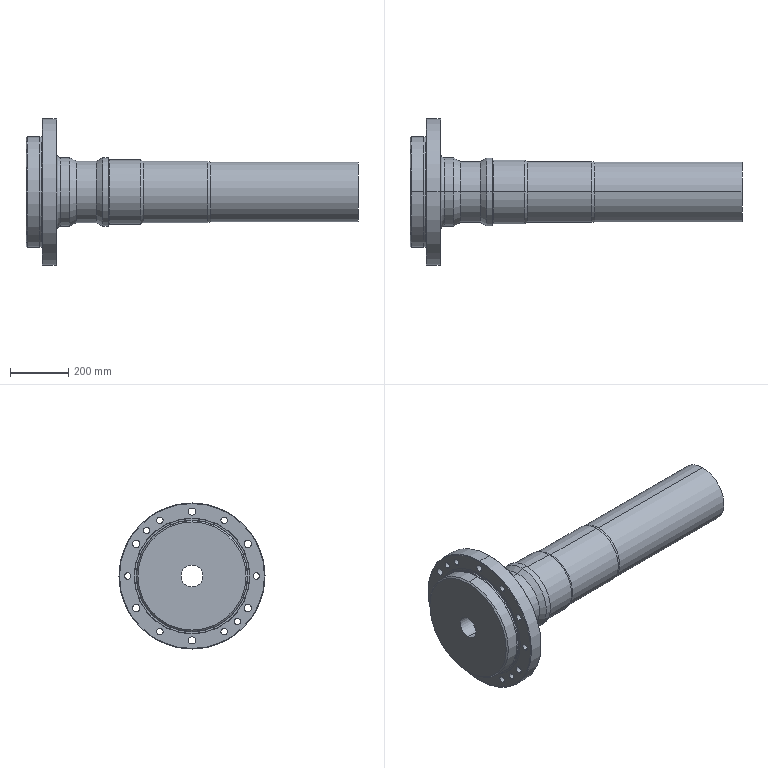Part | SolidWorks | features ICE 2, 3DProfileFeature 1, HoleWzd 1, Revolution 1 | 1 solid | 78 faces | box 1136 x 500 x 500 mm | volume 46733705 mm3 | cylinder 48 | cone 18 | torus 6 | plane 6 | commonest cylinder face diameters 22 x16 25 x12 210 x4 75 x2 205 x2 220 x2